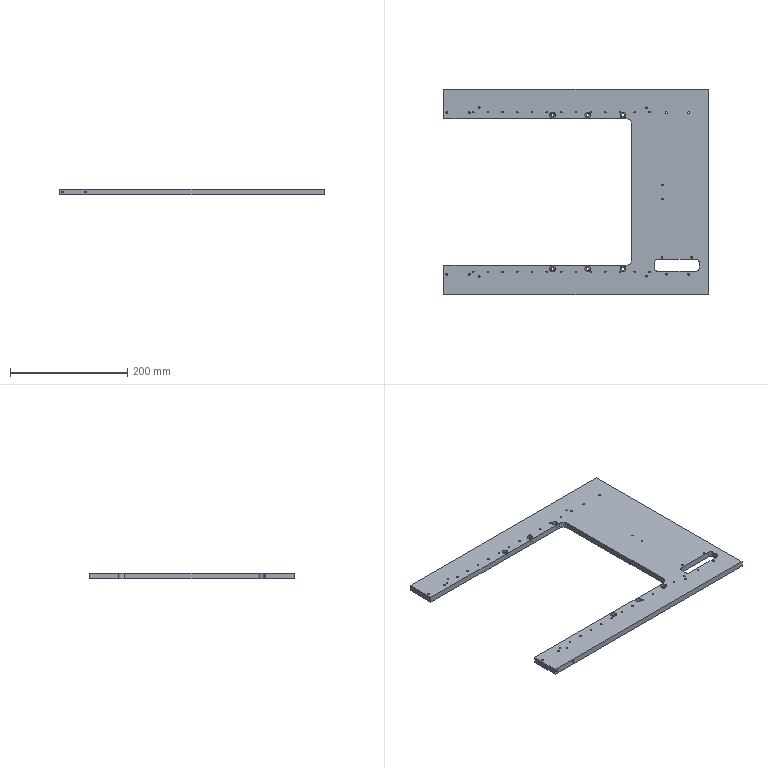Part | SolidWorks | features BaseBody 1 | 1 solid | 150 faces | box 450 x 350 x 10 mm | volume 754366 mm3 | cylinder 122 | plane 20 | cone 8 | commonest cylinder face diameters 2.459 x56 3.242 x28 10 x16 5.5 x12 3 x8 20 x2